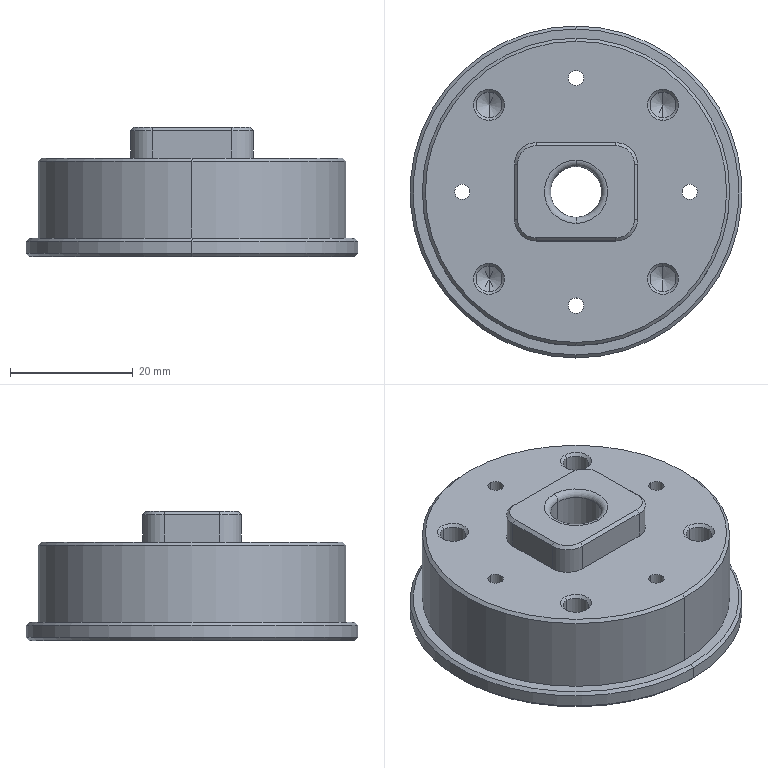NC program | NX | posted with a generic post | part box 54 x 54 x 21 mm
Lines 9361 to 9691 of 9691:
(HOLE_MILLING_1 , TOOL : D3)
N18690 M6
N18692 G54
N18694 G17 G0 G90 X-18.5 Y0. S9500 M3
N18696 G43 Z30. H17
N18698 Z1.
N18700 G94 G3 X-18.7 Y0.2 R0.2 F1250.
N18702 X-18.9 Y0. R0.2
N18704 X-18.9 Y0. Z0.7 I0.4 J0.
N18706 X-18.9 Y0. Z0.4 I0.4 J0.
N18708 X-18.9 Y0. Z0.1 I0.4 J0.
N18710 X-18.9 Y0. Z-0.2 I0.4 J0.
N18712 X-18.9 Y0. Z-0.5 I0.4 J0.
N18714 X-18.9 Y0. Z-0.8 I0.4 J0.
N18716 X-18.9 Y0. Z-1.1 I0.4 J0.
N18718 X-18.9 Y0. Z-1.4 I0.4 J0.
N18720 X-18.9 Y0. Z-1.7 I0.4 J0.
N18722 X-18.9 Y0. Z-2. I0.4 J0.
N18724 X-18.9 Y0. Z-2.3 I0.4 J0.
N18726 X-18.9 Y0. Z-2.6 I0.4 J0.
N18728 X-18.9 Y0. Z-2.9 I0.4 J0.
N18730 X-18.9 Y0. Z-3.2 I0.4 J0.
N18732 X-18.9 Y0. Z-3.5 I0.4 J0.
N18734 X-18.9 Y0. Z-3.8 I0.4 J0.
N18736 X-18.9 Y0. Z-4.1 I0.4 J0.
N18738 X-18.9 Y0. Z-4.4 I0.4 J0.
N18740 X-18.9 Y0. Z-4.7 I0.4 J0.
N18742 X-18.9 Y0. Z-5. I0.4 J0.
N18744 X-18.9 Y0. Z-5.3 I0.4 J0.
N18746 X-18.9 Y0. Z-5.6 I0.4 J0.
N18748 X-18.9 Y0. Z-5.9 I0.4 J0.
N18750 X-18.3 Y-0.346 Z-6. R0.4
N18752 X-18.154 Y0.2 R0.4
N18754 X-18.3 Y-0.346 R-0.4
N18756 X-18.227 Y-0.073 R0.2
N18758 X-18.5 Y0. R0.2
N18760 G0 Z30.
N18762 X0. Y-18.5
N18764 Z1.
N18766 G3 X-0.2 Y-18.3 R0.2
N18768 X-0.4 Y-18.5 R0.2
N18770 X-0.4 Y-18.5 Z0.7 I0.4 J0.
N18772 X-0.4 Y-18.5 Z0.4 I0.4 J0.
N18774 X-0.4 Y-18.5 Z0.1 I0.4 J0.
N18776 X-0.4 Y-18.5 Z-0.2 I0.4 J0.
N18778 X-0.4 Y-18.5 Z-0.5 I0.4 J0.
N18780 X-0.4 Y-18.5 Z-0.8 I0.4 J0.
N18782 X-0.4 Y-18.5 Z-1.1 I0.4 J0.
N18784 X-0.4 Y-18.5 Z-1.4 I0.4 J0.
N18786 X-0.4 Y-18.5 Z-1.7 I0.4 J0.
N18788 X-0.4 Y-18.5 Z-2. I0.4 J0.
N18790 X-0.4 Y-18.5 Z-2.3 I0.4 J0.
N18792 X-0.4 Y-18.5 Z-2.6 I0.4 J0.
N18794 X-0.4 Y-18.5 Z-2.9 I0.4 J0.
N18796 X-0.4 Y-18.5 Z-3.2 I0.4 J0.
N18798 X-0.4 Y-18.5 Z-3.5 I0.4 J0.
N18800 X-0.4 Y-18.5 Z-3.8 I0.4 J0.
N18802 X-0.4 Y-18.5 Z-4.1 I0.4 J0.
N18804 X-0.4 Y-18.5 Z-4.4 I0.4 J0.
N18806 X-0.4 Y-18.5 Z-4.7 I0.4 J0.
N18808 X-0.4 Y-18.5 Z-5. I0.4 J0.
N18810 X-0.4 Y-18.5 Z-5.3 I0.4 J0.
N18812 X-0.4 Y-18.5 Z-5.6 I0.4 J0.
N18814 X-0.4 Y-18.5 Z-5.9 I0.4 J0.
N18816 X0.2 Y-18.846 Z-6. R0.4
N18818 X0.346 Y-18.3 R0.4
N18820 X0.2 Y-18.846 R-0.4
N18822 X0.273 Y-18.573 R0.2
N18824 X0. Y-18.5 R0.2
N18826 G0 Z30.
N18828 X18.5 Y0.
N18830 Z1.
N18832 G3 X18.3 Y0.2 R0.2
N18834 X18.1 Y0. R0.2
N18836 X18.1 Y0. Z0.7 I0.4 J0.
N18838 X18.1 Y0. Z0.4 I0.4 J0.
N18840 X18.1 Y0. Z0.1 I0.4 J0.
N18842 X18.1 Y0. Z-0.2 I0.4 J0.
N18844 X18.1 Y0. Z-0.5 I0.4 J0.
N18846 X18.1 Y0. Z-0.8 I0.4 J0.
N18848 X18.1 Y0. Z-1.1 I0.4 J0.
N18850 X18.1 Y0. Z-1.4 I0.4 J0.
N18852 X18.1 Y0. Z-1.7 I0.4 J0.
N18854 X18.1 Y0. Z-2. I0.4 J0.
N18856 X18.1 Y0. Z-2.3 I0.4 J0.
N18858 X18.1 Y0. Z-2.6 I0.4 J0.
N18860 X18.1 Y0. Z-2.9 I0.4 J0.
N18862 X18.1 Y0. Z-3.2 I0.4 J0.
N18864 X18.1 Y0. Z-3.5 I0.4 J0.
N18866 X18.1 Y0. Z-3.8 I0.4 J0.
N18868 X18.1 Y0. Z-4.1 I0.4 J0.
N18870 X18.1 Y0. Z-4.4 I0.4 J0.
N18872 X18.1 Y0. Z-4.7 I0.4 J0.
N18874 X18.1 Y0. Z-5. I0.4 J0.
N18876 X18.1 Y0. Z-5.3 I0.4 J0.
N18878 X18.1 Y0. Z-5.6 I0.4 J0.
N18880 X18.1 Y0. Z-5.9 I0.4 J0.
N18882 X18.7 Y-0.346 Z-6. R0.4
N18884 X18.846 Y0.2 R0.4
N18886 X18.7 Y-0.346 R-0.4
N18888 X18.773 Y-0.073 R0.2
N18890 X18.5 Y0. R0.2
N18892 G0 Z30.
N18894 X0. Y18.5
N18896 Z1.
N18898 G3 X-0.2 Y18.7 R0.2
N18900 X-0.4 Y18.5 R0.2
N18902 X-0.4 Y18.5 Z0.7 I0.4 J0.
N18904 X-0.4 Y18.5 Z0.4 I0.4 J0.
N18906 X-0.4 Y18.5 Z0.1 I0.4 J0.
N18908 X-0.4 Y18.5 Z-0.2 I0.4 J0.
N18910 X-0.4 Y18.5 Z-0.5 I0.4 J0.
N18912 X-0.4 Y18.5 Z-0.8 I0.4 J0.
N18914 X-0.4 Y18.5 Z-1.1 I0.4 J0.
N18916 X-0.4 Y18.5 Z-1.4 I0.4 J0.
N18918 X-0.4 Y18.5 Z-1.7 I0.4 J0.
N18920 X-0.4 Y18.5 Z-2. I0.4 J0.
N18922 X-0.4 Y18.5 Z-2.3 I0.4 J0.
N18924 X-0.4 Y18.5 Z-2.6 I0.4 J0.
N18926 X-0.4 Y18.5 Z-2.9 I0.4 J0.
N18928 X-0.4 Y18.5 Z-3.2 I0.4 J0.
N18930 X-0.4 Y18.5 Z-3.5 I0.4 J0.
N18932 X-0.4 Y18.5 Z-3.8 I0.4 J0.
N18934 X-0.4 Y18.5 Z-4.1 I0.4 J0.
N18936 X-0.4 Y18.5 Z-4.4 I0.4 J0.
N18938 X-0.4 Y18.5 Z-4.7 I0.4 J0.
N18940 X-0.4 Y18.5 Z-5. I0.4 J0.
N18942 X-0.4 Y18.5 Z-5.3 I0.4 J0.
N18944 X-0.4 Y18.5 Z-5.6 I0.4 J0.
N18946 X-0.4 Y18.5 Z-5.9 I0.4 J0.
N18948 X0.2 Y18.154 Z-6. R0.4
N18950 X0.346 Y18.7 R0.4
N18952 X0.2 Y18.154 R-0.4
N18954 X0.273 Y18.427 R0.2
N18956 X0. Y18.5 R0.2
N18958 G0 Z30.
N18960 M5
(PLANAR_MILL_COPY_COPY_COPY_COPY_COPY_COPY_1_COPY_1 , TOOL : D6A45)
N18962 T01 M6
N18964 G54
N18966 G17 G0 G90 X19. Y-0.866 S9500 M3
N18968 G43 Z30. H1
N18970 Z0.
N18972 G94 G1 Z-1.5 F1250.
N18974 G3 X19.5 Y0. R1.
N18976 X18.5 Y1. R1.
N18978 X19.5 Y0. R-1.
N18980 X19. Y0.866 R1.
N18982 G1 Z0.
N18984 G0 Z30.
N18986 X-0.866 Y-19.
N18988 Z0.
N18990 G1 Z-1.5
N18992 G3 X0. Y-19.5 R1.
N18994 X1. Y-18.5 R1.
N18996 X0. Y-19.5 R-1.
N18998 X0.866 Y-19. R1.
N19000 G1 Z0.
N19002 G0 Z30.
N19004 Y-28.5
N19006 Z0.
N19008 G1 Z-1.5
N19010 G3 X0. Y-28. R1.
N19012 G2 X-28. Y0. R28.
N19014 X0. Y-28. R-28.
N19016 G3 X-0.866 Y-28.5 R1.
N19018 G1 Z0.
N19020 G0 Z30.
N19022 X-19. Y0.866
N19024 Z0.
N19026 G1 Z-1.5
N19028 G3 X-19.5 Y0. R1.
N19030 X-18.5 Y-1. R1.
N19032 X-19.5 Y0. R-1.
N19034 X-19. Y-0.866 R1.
N19036 G1 Z0.
N19038 G0 Z30.
N19040 X-16.36 Y-5.153
N19042 Z0.
N19044 G1 Z-1.5
N19046 G3 X-17.352 Y-5.023 R1.
N19048 G1 X-19.243 Y-5.806
N19050 G3 X-20.325 Y-8.419 R2.
N19052 X-17.712 Y-9.501 R2.
N19054 G1 X-13.93 Y-7.935
N19056 G2 X-9.482 Y-8.894 R4.
N19058 G3 X-8.894 Y-9.482 R13.
N19060 G2 X-7.935 Y-13.93 R4.
N19062 G1 X-9.501 Y-17.712
N19064 G3 X-8.419 Y-20.325 R2.
N19066 X-5.806 Y-19.243 R2.
N19068 G1 X-4.239 Y-15.461
N19070 G2 X-0.416 Y-12.993 R4.
N19072 G3 X0.416 Y-12.993 R13.
N19074 G2 X4.239 Y-15.461 R4.
N19076 G1 X5.806 Y-19.243
N19078 G3 X8.419 Y-20.325 R2.
N19080 X9.501 Y-17.712 R2.
N19082 G1 X7.935 Y-13.93
N19084 G2 X8.894 Y-9.482 R4.
N19086 G3 X9.482 Y-8.894 R13.
N19088 G2 X13.93 Y-7.935 R4.
N19090 G1 X17.712 Y-9.501
N19092 G3 X20.325 Y-8.419 R2.
N19094 X19.243 Y-5.806 R2.
N19096 G1 X15.461 Y-4.239
N19098 G2 X12.993 Y-0.416 R4.
N19100 G3 X12.993 Y0.416 R13.
N19102 G2 X15.461 Y4.239 R4.
N19104 G1 X19.243 Y5.806
N19106 G3 X20.325 Y8.419 R2.
N19108 X17.712 Y9.501 R2.
N19110 G1 X13.93 Y7.935
N19112 G2 X9.482 Y8.894 R4.
N19114 G3 X8.894 Y9.482 R13.
N19116 G2 X7.935 Y13.93 R4.
N19118 G1 X9.501 Y17.712
N19120 G3 X8.419 Y20.325 R2.
N19122 X5.806 Y19.243 R2.
N19124 G1 X4.239 Y15.461
N19126 G2 X0.416 Y12.993 R4.
N19128 G3 X-0.416 Y12.993 R13.
N19130 G2 X-4.239 Y15.461 R4.
N19132 G1 X-5.806 Y19.243
N19134 G3 X-8.419 Y20.325 R2.
N19136 X-9.501 Y17.712 R2.
N19138 G1 X-7.935 Y13.93
N19140 G2 X-8.894 Y9.482 R4.
N19142 G3 X-9.482 Y8.894 R13.
N19144 G2 X-13.93 Y7.935 R4.
N19146 G1 X-17.712 Y9.501
N19148 G3 X-20.325 Y8.419 R2.
N19150 X-19.243 Y5.806 R2.
N19152 G1 X-15.461 Y4.239
N19154 G2 X-12.993 Y0.416 R4.
N19156 G3 X-12.993 Y-0.416 R13.
N19158 G2 X-15.461 Y-4.239 R4.
N19160 G1 X-17.352 Y-5.023
N19162 G3 X-17.961 Y-5.816 R1.
N19164 G1 Z0.
N19166 G0 Z30.
N19168 X0.866 Y19.
N19170 Z0.
N19172 G1 Z-1.5
N19174 G3 X0. Y19.5 R1.
N19176 X-1. Y18.5 R1.
N19178 X0. Y19.5 R-1.
N19180 X-0.866 Y19. R1.
N19182 G1 Z0.
N19184 G0 Z30.
(PLANAR_MILL_COPY_COPY_COPY_COPY_COPY_COPY_1_COPY_1_COPY , TOOL : D6A45)
N19186 X0.866 Y2.75
N19188 Z-1.5
N19190 G1 Z-3.
N19192 G3 X0. Y3.25 R1.
N19194 X-3.25 Y0. R3.25
N19196 X0. Y3.25 R-3.25
N19198 X-0.866 Y2.75 R1.
N19200 G1 Z-1.5
N19202 G0 Z30.
N19204 M5
(CUTTERCOMP , TOOL : D3)
N19206 T17 M6
N19208 G54
N19210 G17 G0 G90 X-18.5 Y0. S9500 M3
N19212 G43 Z30. H17
N19214 Z1.
N19216 G41 G94 G1 X-18.527 Y0.096 F1250. D17
N19218 G3 X-18.95 Y0. R0.222
N19220 X-18.95 Y0. Z-1. I0.45 J0.
N19222 X-18.95 Y0. Z-3. I0.45 J0.
N19224 X-18.95 Y0. Z-5. I0.45 J0.
N19226 X-18.05 Y0. Z-6. I0.45 J0.
N19228 X-18.5 Y0.45 R0.45
N19230 X-18.05 Y0. R-0.45
N19232 X-18.473 Y0.096 R0.222
N19234 G40
N19236 G1 X-18.5 Y0.
N19238 G0 Z30.
N19240 X0. Y-18.5
N19242 Z1.
N19244 G41 G1 X-0.027 Y-18.404
N19246 G3 X-0.45 Y-18.5 R0.222
N19248 X-0.45 Y-18.5 Z-1. I0.45 J0.
N19250 X-0.45 Y-18.5 Z-3. I0.45 J0.
N19252 X-0.45 Y-18.5 Z-5. I0.45 J0.
N19254 X0.45 Y-18.5 Z-6. I0.45 J0.
N19256 X0. Y-18.05 R0.45
N19258 X0.45 Y-18.5 R-0.45
N19260 X0.027 Y-18.404 R0.222
N19262 G40
N19264 G1 X0. Y-18.5
N19266 G0 Z30.
N19268 X18.5 Y0.
N19270 Z1.
N19272 G41 G1 X18.473 Y0.096
N19274 G3 X18.05 Y0. R0.222
N19276 X18.05 Y0. Z-1. I0.45 J0.
N19278 X18.05 Y0. Z-3. I0.45 J0.
N19280 X18.05 Y0. Z-5. I0.45 J0.
N19282 X18.95 Y0. Z-6. I0.45 J0.
N19284 X18.5 Y0.45 R0.45
N19286 X18.95 Y0. R-0.45
N19288 X18.527 Y0.096 R0.222
N19290 G40
N19292 G1 X18.5 Y0.
N19294 G0 Z30.
N19296 X0. Y18.5
N19298 Z1.
N19300 G41 G1 X-0.027 Y18.596
N19302 G3 X-0.45 Y18.5 R0.222
N19304 X-0.45 Y18.5 Z-1. I0.45 J0.
N19306 X-0.45 Y18.5 Z-3. I0.45 J0.
N19308 X-0.45 Y18.5 Z-5. I0.45 J0.
N19310 X0.45 Y18.5 Z-6. I0.45 J0.
N19312 X0. Y18.95 R0.45
N19314 X0.45 Y18.5 R-0.45
N19316 X0.027 Y18.596 R0.222
N19318 G40
N19320 G1 X0. Y18.5
N19322 G0 Z30.
N19324 M5
N19326 M2